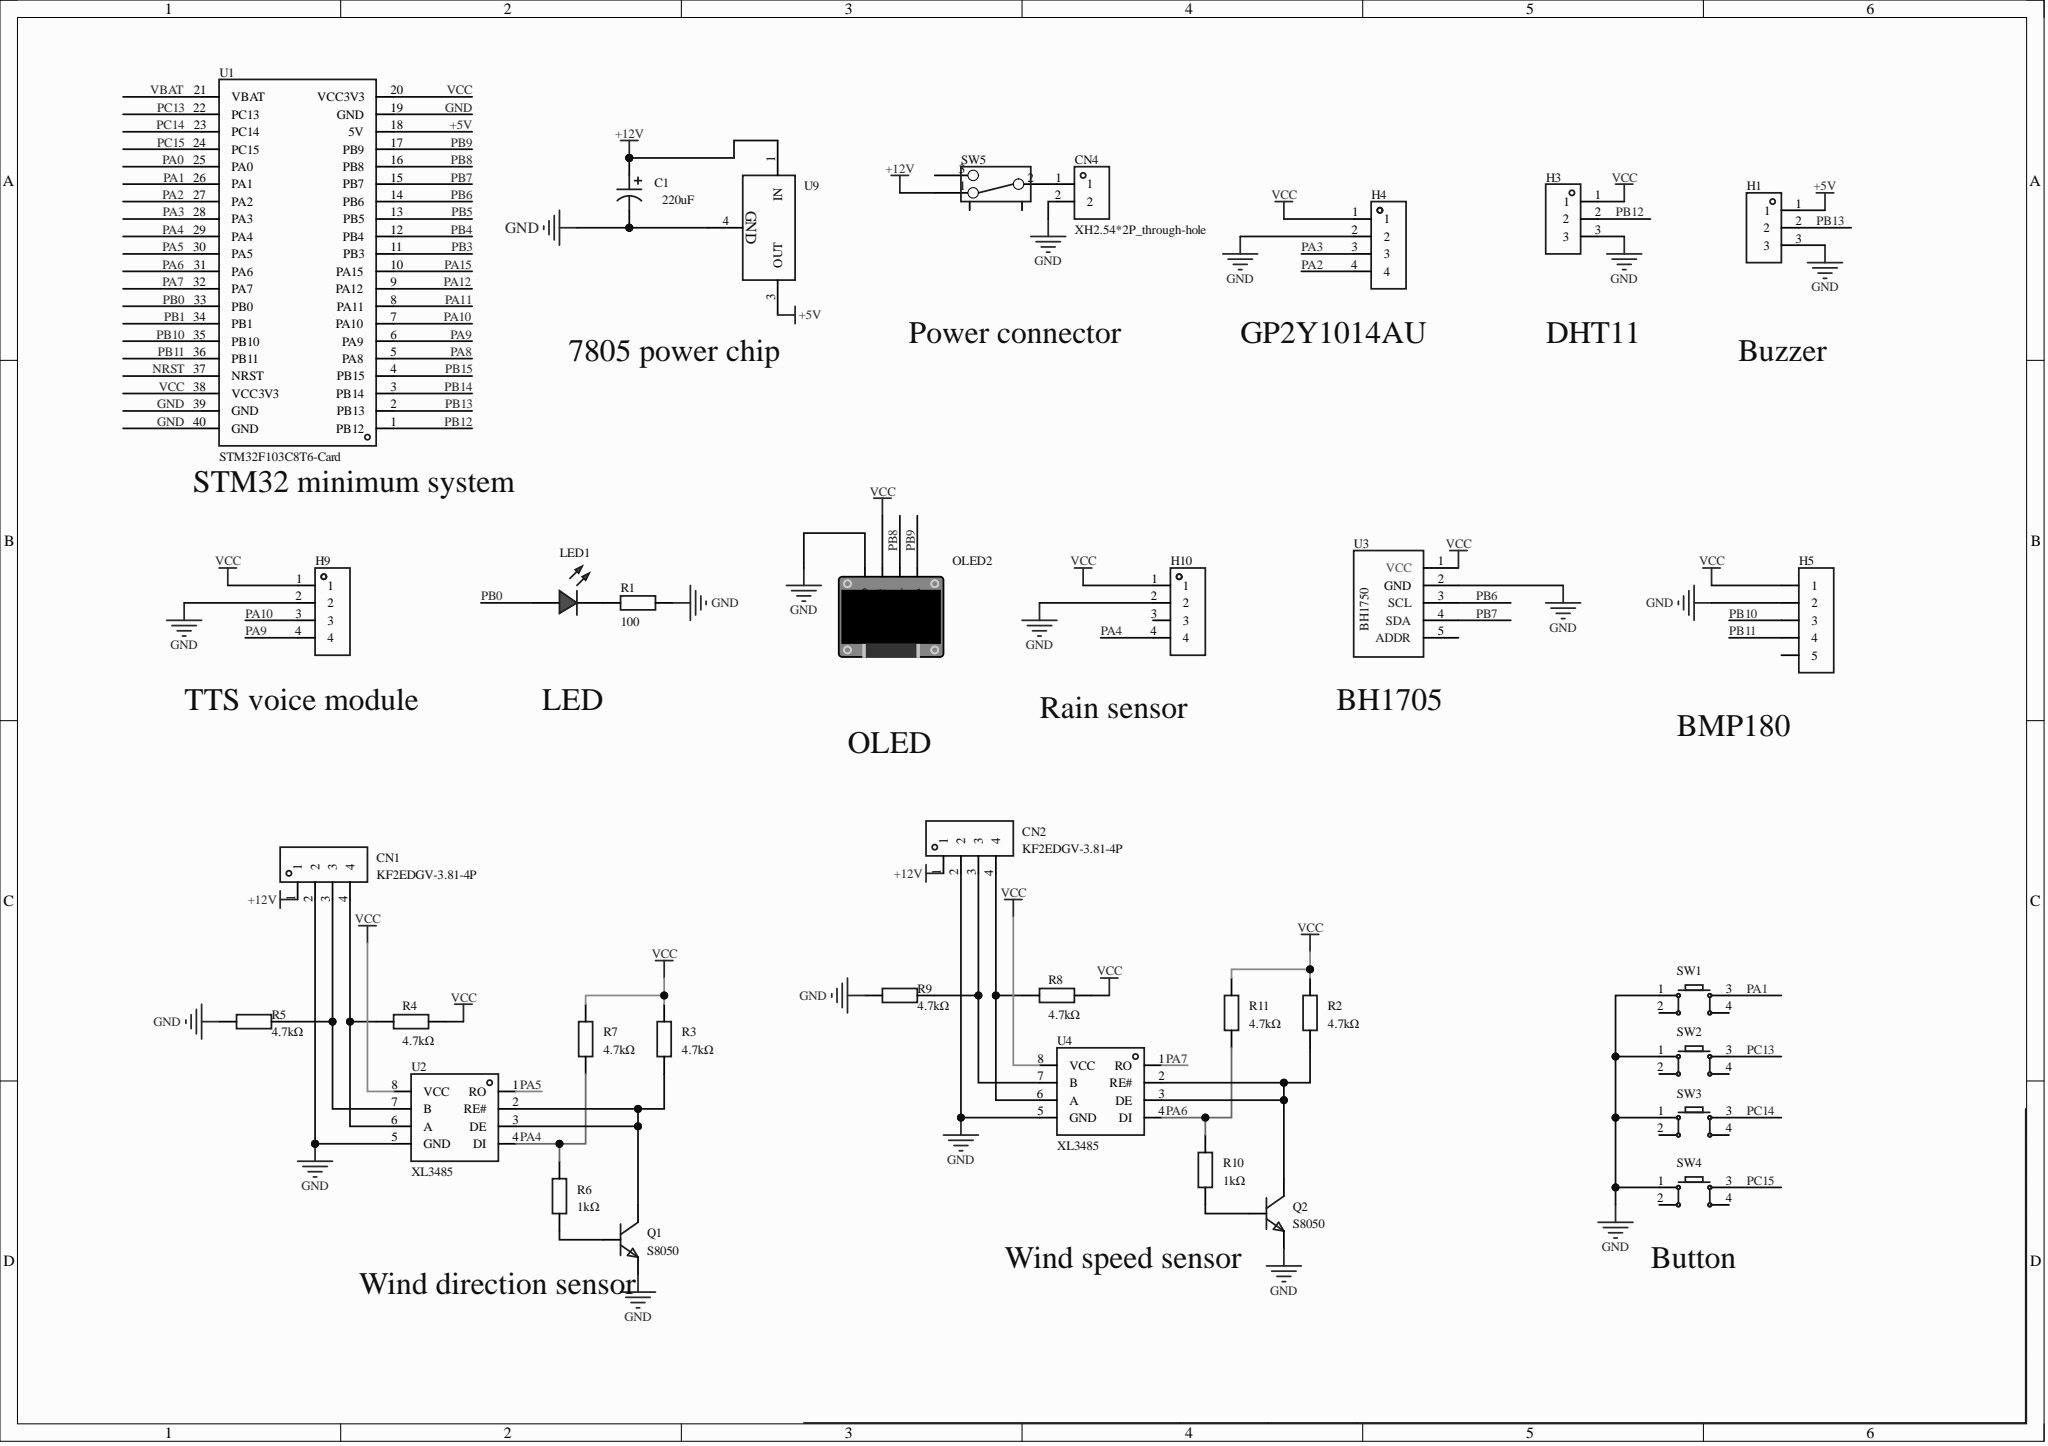Circuit board | Altium Designer | 35 parts | 35 nets
Bill of materials:
Comment,Description,Designator,Footprint,LibRef,Quantity
"","容值:220uF;精度:±20%;额定电压:35V;电容体直径:-;电容体长度:-;纹波电流:-;等效串联电阻:-;工作寿命:-;工作温度:-;","C1","CAP-SMD_BD8.0-L8.3-W8.3-LS9.3-FD","EMK1VM221FB0D00R","1"
"KF2EDGV-3.81-4P","","CN1, CN2","CONN-TH_4P-P3.81_KF2EDGV-3.81-4P","KF2EDGV-3.81-4P","2"
"XH2.54*2P_through-hole","","CN4","CONN-TH_2P-P2.50-XH2.54-2P","XH2.54*2P_直插","1"
"","","H1, H3","HDR-TH_3P-P2.54-V-F","HDR-F_2.54_1x3P","2"
"","","H4, H9, H10","HDR-TH_4P-P2.54-V-F","HDR-F_2.54_1x4P","3"
"","","H5","HDR-TH_5P-P2.54-V-F","HDR-F_2.54_1x5P","1"
"","","LED1","LED_TH-3mm","LED_TH-R_3mm","1"
"","","OLED2","0.96OLED_4P","0.96OLED模块_4P","1"
"S8050","","Q1, Q2","SOT-523-3_L1.6-W0.8-P0.50-LS1.6-BR","S8050_C19630847","2"
"100","","R1","Res_1/8W","Res_AXIAL-1/8W","1"
"4.7kΩ","","R2, R3, R4, R5, R7, R8, R9, R11","R0402ST","R0402S (私有库)","8"
"1kΩ","","R6, R10","R0402ST","R0402S (私有库)","2"
"","","SW1, SW2, SW3, SW4","SW-TH_4P-L6.0-W6.0-P4.50-LS6.5","Key_TH_6x6x6","4"
"","","SW5","拨动开关","拨动开关_正","1"
"STM32F103C8T6-Card","","U1","CONN-TH_L53.3-W22.9_STM32F103C8T6-CARD","STM32F103C8T6-Card","1"
"XL3485","收发器 驱动器/接收器：1/1 数据速率：10Mbps 电源电压：3V~3.6V","U2, U4","SOP-8_L5.0-W4.0-P1.27-LS6.0-BL","XL3485","2"
"","","U3","BH1750光照传感器","BH1750光照传感器","1"
"L78M05ABDT-TR","L78M Series 500 mA 5 V Three Terminal Positive Voltage LDO Regulator - TO-252","U9","TO-252-2_L6.5-W6.1-P4.58-LS10.0-TL","L78M05ABDT-TR","1"
Netlist (Protel format):
[
C1
CAP-SMD_BD8.0-L8.3-W8.3-LS9.3-FD




]
[
CN1
CONN-TH_4P-P3.81_KF2EDGV-3.81-4P
KF2EDGV-3.81-4P



]
[
CN2
CONN-TH_4P-P3.81_KF2EDGV-3.81-4P
KF2EDGV-3.81-4P



]
[
CN4
CONN-TH_2P-P2.50-XH2.54-2P
XH2.54*2P_through-hole



]
[
H1
HDR-TH_3P-P2.54-V-F




]
[
H3
HDR-TH_3P-P2.54-V-F




]
[
H4
HDR-TH_4P-P2.54-V-F




]
[
H5
HDR-TH_5P-P2.54-V-F




]
[
H9
HDR-TH_4P-P2.54-V-F




]
[
H10
HDR-TH_4P-P2.54-V-F




]
[
LED1
LED_TH-3mm




]
[
OLED2
0.96OLED_4P




]
[
Q1
SOT-523-3_L1.6-W0.8-P0.50-LS1.6-BR
S8050



]
[
Q2
SOT-523-3_L1.6-W0.8-P0.50-LS1.6-BR
S8050



]
[
R1
Res_1/8W
100



]
[
R2
R0402ST
4.7kΩ



]
[
R3
R0402ST
4.7kΩ



]
[
R4
R0402ST
4.7kΩ



]
[
R5
R0402ST
4.7kΩ



]
[
R6
R0402ST
1kΩ



]
[
R7
R0402ST
4.7kΩ



]
[
R8
R0402ST
4.7kΩ



]
[
R9
R0402ST
4.7kΩ



]
[
R10
R0402ST
1kΩ



]
[
R11
R0402ST
4.7kΩ



]
[
SW1
SW-TH_4P-L6.0-W6.0-P4.50-LS6.5




]
[
SW2
SW-TH_4P-L6.0-W6.0-P4.50-LS6.5




]
[
SW3
SW-TH_4P-L6.0-W6.0-P4.50-LS6.5




]
[
SW4
SW-TH_4P-L6.0-W6.0-P4.50-LS6.5




]
[
SW5
拨动开关




]
[
U1
CONN-TH_L53.3-W22.9_STM32F103C8T6-CARD
STM32F103C8T6-Card



]
[
U2
SOP-8_L5.0-W4.0-P1.27-LS6.0-BL
XL3485



]
[
U3
BH1750光照传感器




]
[
U4
SOP-8_L5.0-W4.0-P1.27-LS6.0-BL
XL3485



]
[
U9
TO-252-2_L6.5-W6.1-P4.58-LS10.0-TL
L78M05ABDT-TR



]
(
VCC
H3-1
H4-1
H5-1
H9-1
H10-1
OLED2-2
R2-1
R3-1
R4-2
R7-1
R8-2
R11-1
U1-20
U1-38
U2-8
U3-1
U4-8
)
(
PC15
SW4-3
U1-24
)
(
PC14
SW3-3
U1-23
)
(
PC13
SW2-3
U1-22
)
(
PB13
H1-2
U1-2
)
(
PB12
H3-2
U1-1
)
(
PB11
H5-4
U1-36
)
(
PB10
H5-3
U1-35
)
(
PB9
OLED2-4
U1-17
)
(
PB8
OLED2-3
U1-16
)
(
PB7
U1-15
U3-4
)
(
PB6
U1-14
U3-3
)
(
PB0
LED1-1
U1-33
)
(
PA10
H9-3
U1-7
)
(
PA9
H9-4
U1-6
)
(
PA7
U1-32
U4-1
)
(
PA6
R10-2
R11-2
U1-31
U4-4
)
(
PA5
U1-30
U2-1
)
(
PA4
H10-4
R6-2
R7-2
U1-29
U2-4
)
(
PA3
H4-3
U1-28
)
(
PA2
H4-4
U1-27
)
(
PA1
SW1-3
U1-26
)
(
NetQ2_3
Q2-3
R2-2
U4-2
U4-3
)
(
NetQ2_1
Q2-1
R10-1
)
(
NetQ1_3
Q1-3
R3-2
U2-2
U2-3
)
(
NetQ1_1
Q1-1
R6-1
)
(
NetLED1_2
LED1-2
R1-1
)
(
NetCN4_1
CN4-1
SW5-2
)
(
NetCN2_4
CN2-4
R8-1
U4-6
)
(
NetCN2_3
CN2-3
R9-2
U4-7
)
(
NetCN1_4
CN1-4
R4-1
U2-6
)
(
NetCN1_3
CN1-3
R5-2
U2-7
)
(
GND
C1-2
CN1-2
CN2-2
CN4-2
H1-3
H3-3
H4-2
H5-2
H9-2
H10-2
OLED2-1
Q1-2
Q2-2
R1-2
R5-1
R9-1
SW1-1
SW2-1
SW3-1
SW4-1
U1-19
U1-39
U1-40
U2-5
U3-2
U4-5
U9-4
)
(
+12V
C1-1
CN1-1
CN2-1
SW5-1
U9-1
)
(
+5V
H1-1
U1-18
U9-3
)